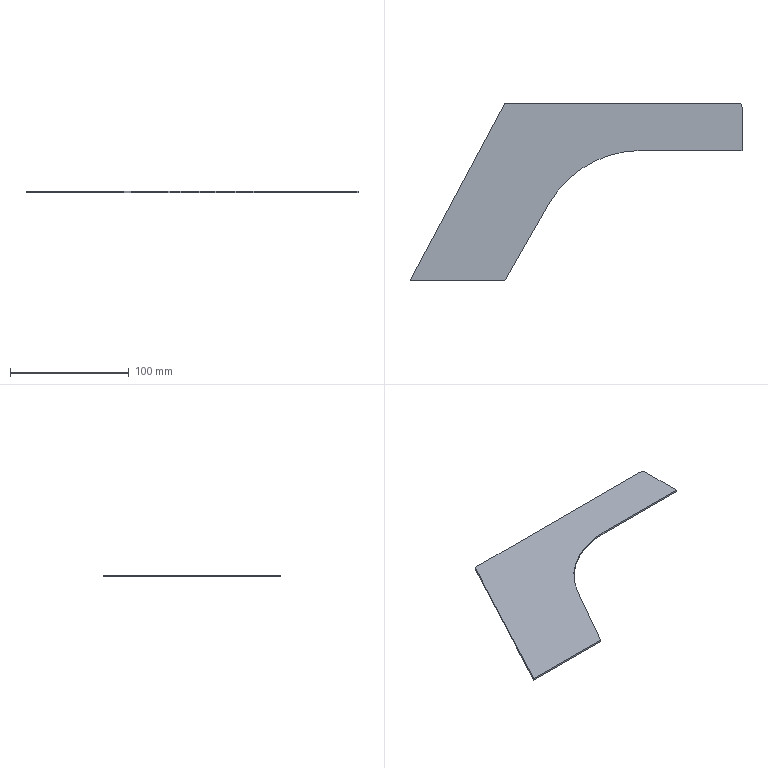Part | SolidWorks | features Extrusion 1 | 1 solid | 11 faces | box 280 x 150 x 1.5 mm | volume 26833 mm3 | plane 8 | cylinder 3 | commonest cylinder face diameters 7 x2 180 x1
STEP:
#1=CARTESIAN_POINT('',(80.,0.,0.));
#2=VERTEX_POINT('',#1);
#3=CARTESIAN_POINT('',(116.813,64.574,0.));
#4=VERTEX_POINT('',#3);
#5=CARTESIAN_POINT('',(80.,0.,0.));
#6=DIRECTION('',(0.4953,0.8687,0.));
#7=VECTOR('',#6,1000.);
#8=LINE('',#5,#7);
#9=EDGE_CURVE('',#2,#4,#8,.T.);
#10=ORIENTED_EDGE('',*,*,#9,.T.);
#11=CARTESIAN_POINT('',(116.813,64.574,1.5));
#12=VERTEX_POINT('',#11);
#13=CARTESIAN_POINT('',(116.813,64.574,1.5));
#14=DIRECTION('',(0.,0.,-1.));
#15=VECTOR('',#14,1000.);
#16=LINE('',#13,#15);
#17=EDGE_CURVE('',#12,#4,#16,.T.);
#18=ORIENTED_EDGE('',*,*,#17,.F.);
#19=CARTESIAN_POINT('',(80.,0.,1.5));
#20=VERTEX_POINT('',#19);
#21=CARTESIAN_POINT('',(80.,0.,1.5));
#22=DIRECTION('',(0.4953,0.8687,0.));
#23=VECTOR('',#22,1000.);
#24=LINE('',#21,#23);
#25=EDGE_CURVE('',#20,#12,#24,.T.);
#26=ORIENTED_EDGE('',*,*,#25,.F.);
#27=CARTESIAN_POINT('',(80.,0.,1.5));
#28=DIRECTION('',(0.,0.,-1.));
#29=VECTOR('',#28,1000.);
#30=LINE('',#27,#29);
#31=EDGE_CURVE('',#20,#2,#30,.T.);
#32=ORIENTED_EDGE('',*,*,#31,.T.);
#33=EDGE_LOOP('',(#10,#18,#26,#32));
#34=FACE_OUTER_BOUND('',#33,.T.);
#35=CARTESIAN_POINT('',(80.,0.,1.5));
#36=DIRECTION('',(-0.8687,0.4953,0.));
#37=DIRECTION('',(-0.4953,-0.8687,0.));
#38=AXIS2_PLACEMENT_3D('',#35,#36,#37);
#39=PLANE('',#38);
#40=ADVANCED_FACE('',(#34),#39,.F.);
#41=CARTESIAN_POINT('',(195.,110.,0.));
#42=VERTEX_POINT('',#41);
#43=CARTESIAN_POINT('',(195.,20.,0.));
#44=DIRECTION('',(0.,0.,1.));
#45=DIRECTION('',(1.,0.,0.));
#46=AXIS2_PLACEMENT_3D('',#43,#44,#45);
#47=CIRCLE('',#46,90.);
#48=EDGE_CURVE('',#42,#4,#47,.T.);
#49=ORIENTED_EDGE('',*,*,#48,.F.);
#50=CARTESIAN_POINT('',(195.,110.,1.5));
#51=VERTEX_POINT('',#50);
#52=CARTESIAN_POINT('',(195.,110.,1.5));
#53=DIRECTION('',(0.,0.,-1.));
#54=VECTOR('',#53,1000.);
#55=LINE('',#52,#54);
#56=EDGE_CURVE('',#51,#42,#55,.T.);
#57=ORIENTED_EDGE('',*,*,#56,.F.);
#58=CARTESIAN_POINT('',(195.,20.,1.5));
#59=DIRECTION('',(0.,0.,1.));
#60=DIRECTION('',(1.,0.,0.));
#61=AXIS2_PLACEMENT_3D('',#58,#59,#60);
#62=CIRCLE('',#61,90.);
#63=EDGE_CURVE('',#51,#12,#62,.T.);
#64=ORIENTED_EDGE('',*,*,#63,.T.);
#65=ORIENTED_EDGE('',*,*,#17,.T.);
#66=EDGE_LOOP('',(#49,#57,#64,#65));
#67=FACE_OUTER_BOUND('',#66,.T.);
#68=CARTESIAN_POINT('',(195.,20.,1.5));
#69=DIRECTION('',(0.,0.,-1.));
#70=DIRECTION('',(-1.,0.,0.));
#71=AXIS2_PLACEMENT_3D('',#68,#69,#70);
#72=CYLINDRICAL_SURFACE('',#71,90.);
#73=ADVANCED_FACE('',(#67),#72,.F.);
#74=CARTESIAN_POINT('',(280.,110.,0.));
#75=VERTEX_POINT('',#74);
#76=CARTESIAN_POINT('',(195.,110.,0.));
#77=DIRECTION('',(1.,0.,0.));
#78=VECTOR('',#77,1000.);
#79=LINE('',#76,#78);
#80=EDGE_CURVE('',#42,#75,#79,.T.);
#81=ORIENTED_EDGE('',*,*,#80,.T.);
#82=CARTESIAN_POINT('',(280.,110.,1.5));
#83=VERTEX_POINT('',#82);
#84=CARTESIAN_POINT('',(280.,110.,1.5));
#85=DIRECTION('',(0.,0.,-1.));
#86=VECTOR('',#85,1000.);
#87=LINE('',#84,#86);
#88=EDGE_CURVE('',#83,#75,#87,.T.);
#89=ORIENTED_EDGE('',*,*,#88,.F.);
#90=CARTESIAN_POINT('',(195.,110.,1.5));
#91=DIRECTION('',(1.,0.,0.));
#92=VECTOR('',#91,1000.);
#93=LINE('',#90,#92);
#94=EDGE_CURVE('',#51,#83,#93,.T.);
#95=ORIENTED_EDGE('',*,*,#94,.F.);
#96=ORIENTED_EDGE('',*,*,#56,.T.);
#97=EDGE_LOOP('',(#81,#89,#95,#96));
#98=FACE_OUTER_BOUND('',#97,.T.);
#99=CARTESIAN_POINT('',(195.,110.,1.5));
#100=DIRECTION('',(0.,1.,0.));
#101=DIRECTION('',(0.,0.,1.));
#102=AXIS2_PLACEMENT_3D('',#99,#100,#101);
#103=PLANE('',#102);
#104=ADVANCED_FACE('',(#98),#103,.F.);
#105=CARTESIAN_POINT('',(280.,146.5,0.));
#106=VERTEX_POINT('',#105);
#107=CARTESIAN_POINT('',(280.,146.5,0.));
#108=DIRECTION('',(0.,-1.,0.));
#109=VECTOR('',#108,1000.);
#110=LINE('',#107,#109);
#111=EDGE_CURVE('',#106,#75,#110,.T.);
#112=ORIENTED_EDGE('',*,*,#111,.F.);
#113=CARTESIAN_POINT('',(280.,146.5,1.5));
#114=VERTEX_POINT('',#113);
#115=CARTESIAN_POINT('',(280.,146.5,1.5));
#116=DIRECTION('',(0.,0.,-1.));
#117=VECTOR('',#116,1000.);
#118=LINE('',#115,#117);
#119=EDGE_CURVE('',#114,#106,#118,.T.);
#120=ORIENTED_EDGE('',*,*,#119,.F.);
#121=CARTESIAN_POINT('',(280.,146.5,1.5));
#122=DIRECTION('',(0.,-1.,0.));
#123=VECTOR('',#122,1000.);
#124=LINE('',#121,#123);
#125=EDGE_CURVE('',#114,#83,#124,.T.);
#126=ORIENTED_EDGE('',*,*,#125,.T.);
#127=ORIENTED_EDGE('',*,*,#88,.T.);
#128=EDGE_LOOP('',(#112,#120,#126,#127));
#129=FACE_OUTER_BOUND('',#128,.T.);
#130=CARTESIAN_POINT('',(280.,146.5,1.5));
#131=DIRECTION('',(1.,0.,0.));
#132=DIRECTION('',(0.,1.,0.));
#133=AXIS2_PLACEMENT_3D('',#130,#131,#132);
#134=PLANE('',#133);
#135=ADVANCED_FACE('',(#129),#134,.T.);
#136=CARTESIAN_POINT('',(276.5,150.,0.));
#137=VERTEX_POINT('',#136);
#138=CARTESIAN_POINT('',(276.5,146.5,0.));
#139=DIRECTION('',(0.,0.,-1.));
#140=DIRECTION('',(-1.,0.,0.));
#141=AXIS2_PLACEMENT_3D('',#138,#139,#140);
#142=CIRCLE('',#141,3.5);
#143=EDGE_CURVE('',#137,#106,#142,.T.);
#144=ORIENTED_EDGE('',*,*,#143,.F.);
#145=CARTESIAN_POINT('',(276.5,150.,1.5));
#146=VERTEX_POINT('',#145);
#147=CARTESIAN_POINT('',(276.5,150.,1.5));
#148=DIRECTION('',(0.,0.,-1.));
#149=VECTOR('',#148,1000.);
#150=LINE('',#147,#149);
#151=EDGE_CURVE('',#146,#137,#150,.T.);
#152=ORIENTED_EDGE('',*,*,#151,.F.);
#153=CARTESIAN_POINT('',(276.5,146.5,1.5));
#154=DIRECTION('',(0.,0.,-1.));
#155=DIRECTION('',(-1.,0.,0.));
#156=AXIS2_PLACEMENT_3D('',#153,#154,#155);
#157=CIRCLE('',#156,3.5);
#158=EDGE_CURVE('',#146,#114,#157,.T.);
#159=ORIENTED_EDGE('',*,*,#158,.T.);
#160=ORIENTED_EDGE('',*,*,#119,.T.);
#161=EDGE_LOOP('',(#144,#152,#159,#160));
#162=FACE_OUTER_BOUND('',#161,.T.);
#163=CARTESIAN_POINT('',(276.5,146.5,1.5));
#164=DIRECTION('',(0.,0.,-1.));
#165=DIRECTION('',(-1.,0.,0.));
#166=AXIS2_PLACEMENT_3D('',#163,#164,#165);
#167=CYLINDRICAL_SURFACE('',#166,3.5);
#168=ADVANCED_FACE('',(#162),#167,.T.);
#169=CARTESIAN_POINT('',(82.1,150.,0.));
#170=VERTEX_POINT('',#169);
#171=CARTESIAN_POINT('',(82.1,150.,0.));
#172=DIRECTION('',(1.,0.,0.));
#173=VECTOR('',#172,1000.);
#174=LINE('',#171,#173);
#175=EDGE_CURVE('',#170,#137,#174,.T.);
#176=ORIENTED_EDGE('',*,*,#175,.F.);
#177=CARTESIAN_POINT('',(82.1,150.,1.5));
#178=VERTEX_POINT('',#177);
#179=CARTESIAN_POINT('',(82.1,150.,1.5));
#180=DIRECTION('',(0.,0.,-1.));
#181=VECTOR('',#180,1000.);
#182=LINE('',#179,#181);
#183=EDGE_CURVE('',#178,#170,#182,.T.);
#184=ORIENTED_EDGE('',*,*,#183,.F.);
#185=CARTESIAN_POINT('',(82.1,150.,1.5));
#186=DIRECTION('',(1.,0.,0.));
#187=VECTOR('',#186,1000.);
#188=LINE('',#185,#187);
#189=EDGE_CURVE('',#178,#146,#188,.T.);
#190=ORIENTED_EDGE('',*,*,#189,.T.);
#191=ORIENTED_EDGE('',*,*,#151,.T.);
#192=EDGE_LOOP('',(#176,#184,#190,#191));
#193=FACE_OUTER_BOUND('',#192,.T.);
#194=CARTESIAN_POINT('',(82.1,150.,1.5));
#195=DIRECTION('',(0.,1.,0.));
#196=DIRECTION('',(-1.,0.,0.));
#197=AXIS2_PLACEMENT_3D('',#194,#195,#196);
#198=PLANE('',#197);
#199=ADVANCED_FACE('',(#193),#198,.T.);
#200=CARTESIAN_POINT('',(79.012,148.147,0.));
#201=VERTEX_POINT('',#200);
#202=CARTESIAN_POINT('',(82.1,146.5,0.));
#203=DIRECTION('',(0.,0.,-1.));
#204=DIRECTION('',(-1.,0.,0.));
#205=AXIS2_PLACEMENT_3D('',#202,#203,#204);
#206=CIRCLE('',#205,3.5);
#207=EDGE_CURVE('',#201,#170,#206,.T.);
#208=ORIENTED_EDGE('',*,*,#207,.F.);
#209=CARTESIAN_POINT('',(79.012,148.147,1.5));
#210=VERTEX_POINT('',#209);
#211=CARTESIAN_POINT('',(79.012,148.147,1.5));
#212=DIRECTION('',(0.,0.,-1.));
#213=VECTOR('',#212,1000.);
#214=LINE('',#211,#213);
#215=EDGE_CURVE('',#210,#201,#214,.T.);
#216=ORIENTED_EDGE('',*,*,#215,.F.);
#217=CARTESIAN_POINT('',(82.1,146.5,1.5));
#218=DIRECTION('',(0.,0.,-1.));
#219=DIRECTION('',(-1.,0.,0.));
#220=AXIS2_PLACEMENT_3D('',#217,#218,#219);
#221=CIRCLE('',#220,3.5);
#222=EDGE_CURVE('',#210,#178,#221,.T.);
#223=ORIENTED_EDGE('',*,*,#222,.T.);
#224=ORIENTED_EDGE('',*,*,#183,.T.);
#225=EDGE_LOOP('',(#208,#216,#223,#224));
#226=FACE_OUTER_BOUND('',#225,.T.);
#227=CARTESIAN_POINT('',(82.1,146.5,1.5));
#228=DIRECTION('',(0.,0.,-1.));
#229=DIRECTION('',(-1.,0.,0.));
#230=AXIS2_PLACEMENT_3D('',#227,#228,#229);
#231=CYLINDRICAL_SURFACE('',#230,3.5);
#232=ADVANCED_FACE('',(#226),#231,.T.);
#233=CARTESIAN_POINT('',(0.,0.,0.));
#234=VERTEX_POINT('',#233);
#235=CARTESIAN_POINT('',(0.,0.,0.));
#236=DIRECTION('',(0.4706,0.8824,0.));
#237=VECTOR('',#236,1000.);
#238=LINE('',#235,#237);
#239=EDGE_CURVE('',#234,#201,#238,.T.);
#240=ORIENTED_EDGE('',*,*,#239,.F.);
#241=CARTESIAN_POINT('',(0.,0.,1.5));
#242=VERTEX_POINT('',#241);
#243=CARTESIAN_POINT('',(0.,0.,1.5));
#244=DIRECTION('',(0.,0.,-1.));
#245=VECTOR('',#244,1000.);
#246=LINE('',#243,#245);
#247=EDGE_CURVE('',#242,#234,#246,.T.);
#248=ORIENTED_EDGE('',*,*,#247,.F.);
#249=CARTESIAN_POINT('',(0.,0.,1.5));
#250=DIRECTION('',(0.4706,0.8824,0.));
#251=VECTOR('',#250,1000.);
#252=LINE('',#249,#251);
#253=EDGE_CURVE('',#242,#210,#252,.T.);
#254=ORIENTED_EDGE('',*,*,#253,.T.);
#255=ORIENTED_EDGE('',*,*,#215,.T.);
#256=EDGE_LOOP('',(#240,#248,#254,#255));
#257=FACE_OUTER_BOUND('',#256,.T.);
#258=CARTESIAN_POINT('',(0.,0.,1.5));
#259=DIRECTION('',(-0.8824,0.4706,0.));
#260=DIRECTION('',(-0.4706,-0.8824,0.));
#261=AXIS2_PLACEMENT_3D('',#258,#259,#260);
#262=PLANE('',#261);
#263=ADVANCED_FACE('',(#257),#262,.T.);
#264=CARTESIAN_POINT('',(80.,0.,0.));
#265=DIRECTION('',(-1.,0.,0.));
#266=VECTOR('',#265,1000.);
#267=LINE('',#264,#266);
#268=EDGE_CURVE('',#2,#234,#267,.T.);
#269=ORIENTED_EDGE('',*,*,#268,.F.);
#270=ORIENTED_EDGE('',*,*,#31,.F.);
#271=CARTESIAN_POINT('',(80.,0.,1.5));
#272=DIRECTION('',(-1.,0.,0.));
#273=VECTOR('',#272,1000.);
#274=LINE('',#271,#273);
#275=EDGE_CURVE('',#20,#242,#274,.T.);
#276=ORIENTED_EDGE('',*,*,#275,.T.);
#277=ORIENTED_EDGE('',*,*,#247,.T.);
#278=EDGE_LOOP('',(#269,#270,#276,#277));
#279=FACE_OUTER_BOUND('',#278,.T.);
#280=CARTESIAN_POINT('',(80.,0.,1.5));
#281=DIRECTION('',(0.,-1.,0.));
#282=DIRECTION('',(1.,0.,0.));
#283=AXIS2_PLACEMENT_3D('',#280,#281,#282);
#284=PLANE('',#283);
#285=ADVANCED_FACE('',(#279),#284,.T.);
#286=ORIENTED_EDGE('',*,*,#25,.T.);
#287=ORIENTED_EDGE('',*,*,#63,.F.);
#288=ORIENTED_EDGE('',*,*,#94,.T.);
#289=ORIENTED_EDGE('',*,*,#125,.F.);
#290=ORIENTED_EDGE('',*,*,#158,.F.);
#291=ORIENTED_EDGE('',*,*,#189,.F.);
#292=ORIENTED_EDGE('',*,*,#222,.F.);
#293=ORIENTED_EDGE('',*,*,#253,.F.);
#294=ORIENTED_EDGE('',*,*,#275,.F.);
#295=EDGE_LOOP('',(#286,#287,#288,#289,#290,#291,#292,#293,#294));
#296=FACE_OUTER_BOUND('',#295,.T.);
#297=CARTESIAN_POINT('',(195.,20.,1.5));
#298=DIRECTION('',(0.,0.,1.));
#299=DIRECTION('',(1.,0.,0.));
#300=AXIS2_PLACEMENT_3D('',#297,#298,#299);
#301=PLANE('',#300);
#302=ADVANCED_FACE('',(#296),#301,.T.);
#303=ORIENTED_EDGE('',*,*,#9,.F.);
#304=ORIENTED_EDGE('',*,*,#268,.T.);
#305=ORIENTED_EDGE('',*,*,#239,.T.);
#306=ORIENTED_EDGE('',*,*,#207,.T.);
#307=ORIENTED_EDGE('',*,*,#175,.T.);
#308=ORIENTED_EDGE('',*,*,#143,.T.);
#309=ORIENTED_EDGE('',*,*,#111,.T.);
#310=ORIENTED_EDGE('',*,*,#80,.F.);
#311=ORIENTED_EDGE('',*,*,#48,.T.);
#312=EDGE_LOOP('',(#303,#304,#305,#306,#307,#308,#309,#310,#311));
#313=FACE_OUTER_BOUND('',#312,.T.);
#314=CARTESIAN_POINT('',(195.,20.,0.));
#315=DIRECTION('',(0.,0.,1.));
#316=DIRECTION('',(1.,0.,0.));
#317=AXIS2_PLACEMENT_3D('',#314,#315,#316);
#318=PLANE('',#317);
#319=ADVANCED_FACE('',(#313),#318,.F.);
#320=CLOSED_SHELL('',(#40,#73,#104,#135,#168,#199,#232,#263,#285,#302,#319));
#321=MANIFOLD_SOLID_BREP('',#320);
#322=CARTESIAN_POINT('',(0.,0.,0.));
#323=DIRECTION('',(0.,0.,1.));
#324=DIRECTION('',(1.,0.,0.));
#325=AXIS2_PLACEMENT_3D('',#322,#323,#324);
#326=(LENGTH_UNIT()NAMED_UNIT(*)SI_UNIT(.MILLI.,.METRE.));
#327=UNCERTAINTY_MEASURE_WITH_UNIT(LENGTH_MEASURE(0.00001),#326,'','');
#328=(NAMED_UNIT(*)PLANE_ANGLE_UNIT()SI_UNIT($,.RADIAN.));
#329=(NAMED_UNIT(*)SI_UNIT($,.STERADIAN.)SOLID_ANGLE_UNIT());
#330=(GEOMETRIC_REPRESENTATION_CONTEXT(3)GLOBAL_UNCERTAINTY_ASSIGNED_CONTEXT((#327))GLOBAL_UNIT_ASSIGNED_CONTEXT((#326,#328,#329))REPRESENTATION_CONTEXT('',''));
#331=ADVANCED_BREP_SHAPE_REPRESENTATION('',(#321,#325),#330);